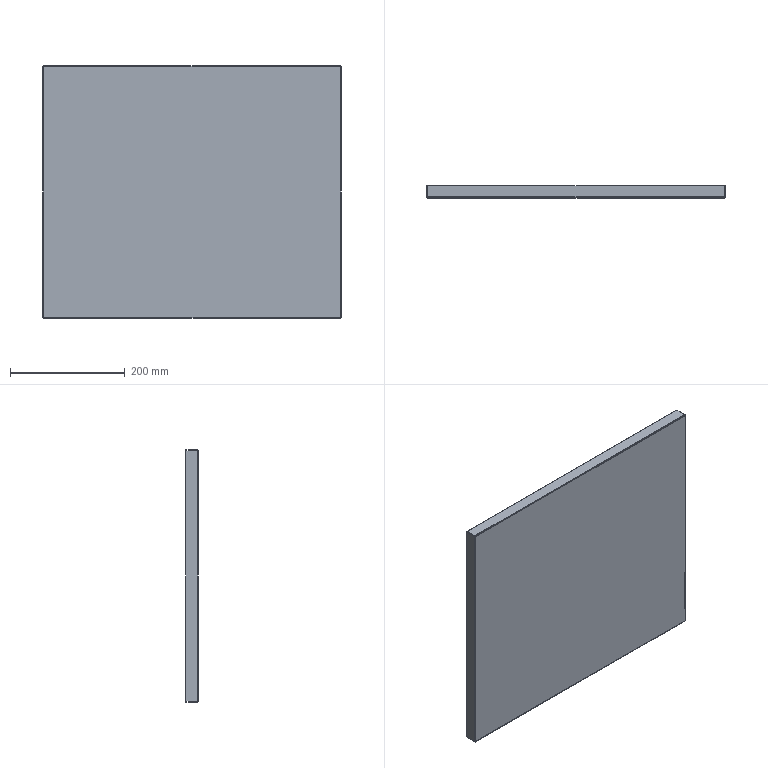Part | SolidWorks | features EdgeFlange 4, FlatPattern 1, SMBaseFlange 1, SheetMetal 1 | 1 solid | 38 faces | box 520 x 21 x 440 mm | volume 266132 mm3 | plane 30 | cylinder 8 | commonest cylinder face diameters 1 x4 3 x4
STEP:
#1=CARTESIAN_POINT('',(-258.5,1.,-218.5));
#2=VERTEX_POINT('',#1);
#3=CARTESIAN_POINT('',(-258.5,1.,218.5));
#4=VERTEX_POINT('',#3);
#5=CARTESIAN_POINT('',(-258.5,1.,-218.5));
#6=DIRECTION('',(0.,0.,1.));
#7=VECTOR('',#6,1000.);
#8=LINE('',#5,#7);
#9=EDGE_CURVE('',#2,#4,#8,.T.);
#10=ORIENTED_EDGE('',*,*,#9,.T.);
#11=CARTESIAN_POINT('',(258.5,1.,218.5));
#12=VERTEX_POINT('',#11);
#13=CARTESIAN_POINT('',(-258.5,1.,218.5));
#14=DIRECTION('',(1.,0.,0.));
#15=VECTOR('',#14,1000.);
#16=LINE('',#13,#15);
#17=EDGE_CURVE('',#4,#12,#16,.T.);
#18=ORIENTED_EDGE('',*,*,#17,.T.);
#19=CARTESIAN_POINT('',(258.5,1.,-218.5));
#20=VERTEX_POINT('',#19);
#21=CARTESIAN_POINT('',(258.5,1.,-218.5));
#22=DIRECTION('',(0.,0.,-1.));
#23=VECTOR('',#22,1000.);
#24=LINE('',#21,#23);
#25=EDGE_CURVE('',#12,#20,#24,.T.);
#26=ORIENTED_EDGE('',*,*,#25,.T.);
#27=CARTESIAN_POINT('',(-258.5,1.,-218.5));
#28=DIRECTION('',(-1.,0.,0.));
#29=VECTOR('',#28,1000.);
#30=LINE('',#27,#29);
#31=EDGE_CURVE('',#20,#2,#30,.T.);
#32=ORIENTED_EDGE('',*,*,#31,.T.);
#33=EDGE_LOOP('',(#10,#18,#26,#32));
#34=FACE_OUTER_BOUND('',#33,.T.);
#35=CARTESIAN_POINT('',(-258.5,1.,218.5));
#36=DIRECTION('',(0.,1.,0.));
#37=DIRECTION('',(0.,0.,1.));
#38=AXIS2_PLACEMENT_3D('',#35,#36,#37);
#39=PLANE('',#38);
#40=ADVANCED_FACE('',(#34),#39,.T.);
#41=CARTESIAN_POINT('',(-258.5,0.,-218.5));
#42=VERTEX_POINT('',#41);
#43=CARTESIAN_POINT('',(-258.5,0.,218.5));
#44=VERTEX_POINT('',#43);
#45=CARTESIAN_POINT('',(-258.5,0.,-218.5));
#46=DIRECTION('',(0.,0.,1.));
#47=VECTOR('',#46,1000.);
#48=LINE('',#45,#47);
#49=EDGE_CURVE('',#42,#44,#48,.T.);
#50=ORIENTED_EDGE('',*,*,#49,.F.);
#51=CARTESIAN_POINT('',(258.5,0.,-218.5));
#52=VERTEX_POINT('',#51);
#53=CARTESIAN_POINT('',(-258.5,0.,-218.5));
#54=DIRECTION('',(-1.,0.,0.));
#55=VECTOR('',#54,1000.);
#56=LINE('',#53,#55);
#57=EDGE_CURVE('',#52,#42,#56,.T.);
#58=ORIENTED_EDGE('',*,*,#57,.F.);
#59=CARTESIAN_POINT('',(258.5,0.,218.5));
#60=VERTEX_POINT('',#59);
#61=CARTESIAN_POINT('',(258.5,0.,-218.5));
#62=DIRECTION('',(0.,0.,-1.));
#63=VECTOR('',#62,1000.);
#64=LINE('',#61,#63);
#65=EDGE_CURVE('',#60,#52,#64,.T.);
#66=ORIENTED_EDGE('',*,*,#65,.F.);
#67=CARTESIAN_POINT('',(-258.5,0.,218.5));
#68=DIRECTION('',(1.,0.,0.));
#69=VECTOR('',#68,1000.);
#70=LINE('',#67,#69);
#71=EDGE_CURVE('',#44,#60,#70,.T.);
#72=ORIENTED_EDGE('',*,*,#71,.F.);
#73=EDGE_LOOP('',(#50,#58,#66,#72));
#74=FACE_OUTER_BOUND('',#73,.T.);
#75=CARTESIAN_POINT('',(-258.5,0.,218.5));
#76=DIRECTION('',(0.,1.,0.));
#77=DIRECTION('',(0.,0.,1.));
#78=AXIS2_PLACEMENT_3D('',#75,#76,#77);
#79=PLANE('',#78);
#80=ADVANCED_FACE('',(#74),#79,.F.);
#81=CARTESIAN_POINT('',(-259.,1.5,-218.5));
#82=VERTEX_POINT('',#81);
#83=CARTESIAN_POINT('',(-260.,1.5,-218.5));
#84=VERTEX_POINT('',#83);
#85=CARTESIAN_POINT('',(-260.,1.5,-218.5));
#86=DIRECTION('',(-1.,0.,0.));
#87=VECTOR('',#86,1000.);
#88=LINE('',#85,#87);
#89=EDGE_CURVE('',#82,#84,#88,.T.);
#90=ORIENTED_EDGE('',*,*,#89,.F.);
#91=CARTESIAN_POINT('',(-258.5,1.5,-218.5));
#92=DIRECTION('',(0.,0.,-1.));
#93=DIRECTION('',(0.,-1.,0.));
#94=AXIS2_PLACEMENT_3D('',#91,#92,#93);
#95=CIRCLE('',#94,0.5);
#96=EDGE_CURVE('',#2,#82,#95,.T.);
#97=ORIENTED_EDGE('',*,*,#96,.F.);
#98=CARTESIAN_POINT('',(-258.5,1.,-218.5));
#99=DIRECTION('',(0.,-1.,0.));
#100=VECTOR('',#99,1000.);
#101=LINE('',#98,#100);
#102=EDGE_CURVE('',#2,#42,#101,.T.);
#103=ORIENTED_EDGE('',*,*,#102,.T.);
#104=CARTESIAN_POINT('',(-258.5,1.5,-218.5));
#105=DIRECTION('',(0.,0.,-1.));
#106=DIRECTION('',(0.,-1.,0.));
#107=AXIS2_PLACEMENT_3D('',#104,#105,#106);
#108=CIRCLE('',#107,1.5);
#109=EDGE_CURVE('',#42,#84,#108,.T.);
#110=ORIENTED_EDGE('',*,*,#109,.T.);
#111=EDGE_LOOP('',(#90,#97,#103,#110));
#112=FACE_OUTER_BOUND('',#111,.T.);
#113=CARTESIAN_POINT('',(-258.5,1.5,-218.5));
#114=DIRECTION('',(0.,0.,-1.));
#115=DIRECTION('',(0.,1.,0.));
#116=AXIS2_PLACEMENT_3D('',#113,#114,#115);
#117=PLANE('',#116);
#118=ADVANCED_FACE('',(#112),#117,.T.);
#119=ORIENTED_EDGE('',*,*,#49,.T.);
#120=CARTESIAN_POINT('',(-260.,1.5,218.5));
#121=VERTEX_POINT('',#120);
#122=CARTESIAN_POINT('',(-258.5,1.5,218.5));
#123=DIRECTION('',(0.,0.,1.));
#124=DIRECTION('',(0.,-1.,0.));
#125=AXIS2_PLACEMENT_3D('',#122,#123,#124);
#126=CIRCLE('',#125,1.5);
#127=EDGE_CURVE('',#121,#44,#126,.T.);
#128=ORIENTED_EDGE('',*,*,#127,.F.);
#129=CARTESIAN_POINT('',(-260.,1.5,-218.5));
#130=DIRECTION('',(0.,0.,-1.));
#131=VECTOR('',#130,1000.);
#132=LINE('',#129,#131);
#133=EDGE_CURVE('',#121,#84,#132,.T.);
#134=ORIENTED_EDGE('',*,*,#133,.T.);
#135=ORIENTED_EDGE('',*,*,#109,.F.);
#136=EDGE_LOOP('',(#119,#128,#134,#135));
#137=FACE_OUTER_BOUND('',#136,.T.);
#138=CARTESIAN_POINT('',(-258.5,1.5,218.5));
#139=DIRECTION('',(0.,0.,1.));
#140=DIRECTION('',(-1.,0.,0.));
#141=AXIS2_PLACEMENT_3D('',#138,#139,#140);
#142=CYLINDRICAL_SURFACE('',#141,1.5);
#143=ADVANCED_FACE('',(#137),#142,.T.);
#144=CARTESIAN_POINT('',(-259.,1.5,218.5));
#145=VERTEX_POINT('',#144);
#146=CARTESIAN_POINT('',(-258.5,1.5,218.5));
#147=DIRECTION('',(0.,0.,1.));
#148=DIRECTION('',(0.,-1.,0.));
#149=AXIS2_PLACEMENT_3D('',#146,#147,#148);
#150=CIRCLE('',#149,0.5);
#151=EDGE_CURVE('',#145,#4,#150,.T.);
#152=ORIENTED_EDGE('',*,*,#151,.F.);
#153=CARTESIAN_POINT('',(-259.,1.5,218.5));
#154=DIRECTION('',(-1.,0.,0.));
#155=VECTOR('',#154,1000.);
#156=LINE('',#153,#155);
#157=EDGE_CURVE('',#145,#121,#156,.T.);
#158=ORIENTED_EDGE('',*,*,#157,.T.);
#159=ORIENTED_EDGE('',*,*,#127,.T.);
#160=CARTESIAN_POINT('',(-258.5,1.,218.5));
#161=DIRECTION('',(0.,-1.,0.));
#162=VECTOR('',#161,1000.);
#163=LINE('',#160,#162);
#164=EDGE_CURVE('',#4,#44,#163,.T.);
#165=ORIENTED_EDGE('',*,*,#164,.F.);
#166=EDGE_LOOP('',(#152,#158,#159,#165));
#167=FACE_OUTER_BOUND('',#166,.T.);
#168=CARTESIAN_POINT('',(-258.5,1.5,218.5));
#169=DIRECTION('',(0.,0.,-1.));
#170=DIRECTION('',(0.,1.,0.));
#171=AXIS2_PLACEMENT_3D('',#168,#169,#170);
#172=PLANE('',#171);
#173=ADVANCED_FACE('',(#167),#172,.F.);
#174=ORIENTED_EDGE('',*,*,#9,.F.);
#175=ORIENTED_EDGE('',*,*,#96,.T.);
#176=CARTESIAN_POINT('',(-259.,1.5,-218.5));
#177=DIRECTION('',(0.,0.,1.));
#178=VECTOR('',#177,1000.);
#179=LINE('',#176,#178);
#180=EDGE_CURVE('',#82,#145,#179,.T.);
#181=ORIENTED_EDGE('',*,*,#180,.T.);
#182=ORIENTED_EDGE('',*,*,#151,.T.);
#183=EDGE_LOOP('',(#174,#175,#181,#182));
#184=FACE_OUTER_BOUND('',#183,.T.);
#185=CARTESIAN_POINT('',(-258.5,1.5,218.5));
#186=DIRECTION('',(0.,0.,1.));
#187=DIRECTION('',(-1.,0.,0.));
#188=AXIS2_PLACEMENT_3D('',#185,#186,#187);
#189=CYLINDRICAL_SURFACE('',#188,0.5);
#190=ADVANCED_FACE('',(#184),#189,.F.);
#191=CARTESIAN_POINT('',(-260.,21.,218.5));
#192=VERTEX_POINT('',#191);
#193=CARTESIAN_POINT('',(-260.,1.,218.5));
#194=DIRECTION('',(0.,-1.,0.));
#195=VECTOR('',#194,1000.);
#196=LINE('',#193,#195);
#197=EDGE_CURVE('',#192,#121,#196,.T.);
#198=ORIENTED_EDGE('',*,*,#197,.T.);
#199=ORIENTED_EDGE('',*,*,#157,.F.);
#200=CARTESIAN_POINT('',(-259.,21.,218.5));
#201=VERTEX_POINT('',#200);
#202=CARTESIAN_POINT('',(-259.,1.,218.5));
#203=DIRECTION('',(0.,-1.,0.));
#204=VECTOR('',#203,1000.);
#205=LINE('',#202,#204);
#206=EDGE_CURVE('',#201,#145,#205,.T.);
#207=ORIENTED_EDGE('',*,*,#206,.F.);
#208=CARTESIAN_POINT('',(-260.,21.,218.5));
#209=DIRECTION('',(1.,0.,0.));
#210=VECTOR('',#209,1000.);
#211=LINE('',#208,#210);
#212=EDGE_CURVE('',#192,#201,#211,.T.);
#213=ORIENTED_EDGE('',*,*,#212,.F.);
#214=EDGE_LOOP('',(#198,#199,#207,#213));
#215=FACE_OUTER_BOUND('',#214,.T.);
#216=CARTESIAN_POINT('',(-260.,1.,218.5));
#217=DIRECTION('',(0.,0.,1.));
#218=DIRECTION('',(0.,-1.,0.));
#219=AXIS2_PLACEMENT_3D('',#216,#217,#218);
#220=PLANE('',#219);
#221=ADVANCED_FACE('',(#215),#220,.T.);
#222=CARTESIAN_POINT('',(-259.,21.,-218.5));
#223=VERTEX_POINT('',#222);
#224=CARTESIAN_POINT('',(-259.,1.,-218.5));
#225=DIRECTION('',(0.,1.,0.));
#226=VECTOR('',#225,1000.);
#227=LINE('',#224,#226);
#228=EDGE_CURVE('',#82,#223,#227,.T.);
#229=ORIENTED_EDGE('',*,*,#228,.F.);
#230=ORIENTED_EDGE('',*,*,#89,.T.);
#231=CARTESIAN_POINT('',(-260.,21.,-218.5));
#232=VERTEX_POINT('',#231);
#233=CARTESIAN_POINT('',(-260.,21.,-218.5));
#234=DIRECTION('',(0.,1.,0.));
#235=VECTOR('',#234,1000.);
#236=LINE('',#233,#235);
#237=EDGE_CURVE('',#84,#232,#236,.T.);
#238=ORIENTED_EDGE('',*,*,#237,.T.);
#239=CARTESIAN_POINT('',(-260.,21.,-218.5));
#240=DIRECTION('',(1.,0.,0.));
#241=VECTOR('',#240,1000.);
#242=LINE('',#239,#241);
#243=EDGE_CURVE('',#232,#223,#242,.T.);
#244=ORIENTED_EDGE('',*,*,#243,.T.);
#245=EDGE_LOOP('',(#229,#230,#238,#244));
#246=FACE_OUTER_BOUND('',#245,.T.);
#247=CARTESIAN_POINT('',(-260.,21.,-218.5));
#248=DIRECTION('',(0.,0.,-1.));
#249=DIRECTION('',(0.,1.,0.));
#250=AXIS2_PLACEMENT_3D('',#247,#248,#249);
#251=PLANE('',#250);
#252=ADVANCED_FACE('',(#246),#251,.T.);
#253=ORIENTED_EDGE('',*,*,#133,.F.);
#254=ORIENTED_EDGE('',*,*,#197,.F.);
#255=CARTESIAN_POINT('',(-260.,21.,218.5));
#256=DIRECTION('',(0.,0.,1.));
#257=VECTOR('',#256,1000.);
#258=LINE('',#255,#257);
#259=EDGE_CURVE('',#232,#192,#258,.T.);
#260=ORIENTED_EDGE('',*,*,#259,.F.);
#261=ORIENTED_EDGE('',*,*,#237,.F.);
#262=EDGE_LOOP('',(#253,#254,#260,#261));
#263=FACE_OUTER_BOUND('',#262,.T.);
#264=CARTESIAN_POINT('',(-260.,1.,-218.5));
#265=DIRECTION('',(1.,0.,0.));
#266=DIRECTION('',(0.,1.,0.));
#267=AXIS2_PLACEMENT_3D('',#264,#265,#266);
#268=PLANE('',#267);
#269=ADVANCED_FACE('',(#263),#268,.F.);
#270=ORIENTED_EDGE('',*,*,#206,.T.);
#271=ORIENTED_EDGE('',*,*,#180,.F.);
#272=ORIENTED_EDGE('',*,*,#228,.T.);
#273=CARTESIAN_POINT('',(-259.,21.,-218.5));
#274=DIRECTION('',(0.,0.,1.));
#275=VECTOR('',#274,1000.);
#276=LINE('',#273,#275);
#277=EDGE_CURVE('',#223,#201,#276,.T.);
#278=ORIENTED_EDGE('',*,*,#277,.T.);
#279=EDGE_LOOP('',(#270,#271,#272,#278));
#280=FACE_OUTER_BOUND('',#279,.T.);
#281=CARTESIAN_POINT('',(-259.,1.,-218.5));
#282=DIRECTION('',(1.,0.,0.));
#283=DIRECTION('',(0.,1.,0.));
#284=AXIS2_PLACEMENT_3D('',#281,#282,#283);
#285=PLANE('',#284);
#286=ADVANCED_FACE('',(#280),#285,.T.);
#287=ORIENTED_EDGE('',*,*,#277,.F.);
#288=ORIENTED_EDGE('',*,*,#243,.F.);
#289=ORIENTED_EDGE('',*,*,#259,.T.);
#290=ORIENTED_EDGE('',*,*,#212,.T.);
#291=EDGE_LOOP('',(#287,#288,#289,#290));
#292=FACE_OUTER_BOUND('',#291,.T.);
#293=CARTESIAN_POINT('',(-260.,21.,218.5));
#294=DIRECTION('',(0.,1.,0.));
#295=DIRECTION('',(-1.,0.,0.));
#296=AXIS2_PLACEMENT_3D('',#293,#294,#295);
#297=PLANE('',#296);
#298=ADVANCED_FACE('',(#292),#297,.T.);
#299=CARTESIAN_POINT('',(259.,1.5,218.5));
#300=VERTEX_POINT('',#299);
#301=CARTESIAN_POINT('',(260.,1.5,218.5));
#302=VERTEX_POINT('',#301);
#303=CARTESIAN_POINT('',(260.,1.5,218.5));
#304=DIRECTION('',(1.,0.,0.));
#305=VECTOR('',#304,1000.);
#306=LINE('',#303,#305);
#307=EDGE_CURVE('',#300,#302,#306,.T.);
#308=ORIENTED_EDGE('',*,*,#307,.F.);
#309=CARTESIAN_POINT('',(258.5,1.5,218.5));
#310=DIRECTION('',(0.,0.,1.));
#311=DIRECTION('',(0.,1.,0.));
#312=AXIS2_PLACEMENT_3D('',#309,#310,#311);
#313=CIRCLE('',#312,0.5);
#314=EDGE_CURVE('',#12,#300,#313,.T.);
#315=ORIENTED_EDGE('',*,*,#314,.F.);
#316=CARTESIAN_POINT('',(258.5,1.,218.5));
#317=DIRECTION('',(0.,-1.,0.));
#318=VECTOR('',#317,1000.);
#319=LINE('',#316,#318);
#320=EDGE_CURVE('',#12,#60,#319,.T.);
#321=ORIENTED_EDGE('',*,*,#320,.T.);
#322=CARTESIAN_POINT('',(258.5,1.5,218.5));
#323=DIRECTION('',(0.,0.,1.));
#324=DIRECTION('',(0.,1.,0.));
#325=AXIS2_PLACEMENT_3D('',#322,#323,#324);
#326=CIRCLE('',#325,1.5);
#327=EDGE_CURVE('',#60,#302,#326,.T.);
#328=ORIENTED_EDGE('',*,*,#327,.T.);
#329=EDGE_LOOP('',(#308,#315,#321,#328));
#330=FACE_OUTER_BOUND('',#329,.T.);
#331=CARTESIAN_POINT('',(258.5,1.5,218.5));
#332=DIRECTION('',(0.,0.,1.));
#333=DIRECTION('',(0.,-1.,0.));
#334=AXIS2_PLACEMENT_3D('',#331,#332,#333);
#335=PLANE('',#334);
#336=ADVANCED_FACE('',(#330),#335,.T.);
#337=ORIENTED_EDGE('',*,*,#65,.T.);
#338=CARTESIAN_POINT('',(260.,1.5,-218.5));
#339=VERTEX_POINT('',#338);
#340=CARTESIAN_POINT('',(258.5,1.5,-218.5));
#341=DIRECTION('',(0.,0.,-1.));
#342=DIRECTION('',(0.,1.,0.));
#343=AXIS2_PLACEMENT_3D('',#340,#341,#342);
#344=CIRCLE('',#343,1.5);
#345=EDGE_CURVE('',#339,#52,#344,.T.);
#346=ORIENTED_EDGE('',*,*,#345,.F.);
#347=CARTESIAN_POINT('',(260.,1.5,-218.5));
#348=DIRECTION('',(0.,0.,-1.));
#349=VECTOR('',#348,1000.);
#350=LINE('',#347,#349);
#351=EDGE_CURVE('',#302,#339,#350,.T.);
#352=ORIENTED_EDGE('',*,*,#351,.F.);
#353=ORIENTED_EDGE('',*,*,#327,.F.);
#354=EDGE_LOOP('',(#337,#346,#352,#353));
#355=FACE_OUTER_BOUND('',#354,.T.);
#356=CARTESIAN_POINT('',(258.5,1.5,-218.5));
#357=DIRECTION('',(0.,0.,-1.));
#358=DIRECTION('',(1.,0.,0.));
#359=AXIS2_PLACEMENT_3D('',#356,#357,#358);
#360=CYLINDRICAL_SURFACE('',#359,1.5);
#361=ADVANCED_FACE('',(#355),#360,.T.);
#362=CARTESIAN_POINT('',(259.,1.5,-218.5));
#363=VERTEX_POINT('',#362);
#364=CARTESIAN_POINT('',(258.5,1.5,-218.5));
#365=DIRECTION('',(0.,0.,-1.));
#366=DIRECTION('',(0.,1.,0.));
#367=AXIS2_PLACEMENT_3D('',#364,#365,#366);
#368=CIRCLE('',#367,0.5);
#369=EDGE_CURVE('',#363,#20,#368,.T.);
#370=ORIENTED_EDGE('',*,*,#369,.F.);
#371=CARTESIAN_POINT('',(259.,1.5,-218.5));
#372=DIRECTION('',(1.,0.,0.));
#373=VECTOR('',#372,1000.);
#374=LINE('',#371,#373);
#375=EDGE_CURVE('',#363,#339,#374,.T.);
#376=ORIENTED_EDGE('',*,*,#375,.T.);
#377=ORIENTED_EDGE('',*,*,#345,.T.);
#378=CARTESIAN_POINT('',(258.5,1.,-218.5));
#379=DIRECTION('',(0.,-1.,0.));
#380=VECTOR('',#379,1000.);
#381=LINE('',#378,#380);
#382=EDGE_CURVE('',#20,#52,#381,.T.);
#383=ORIENTED_EDGE('',*,*,#382,.F.);
#384=EDGE_LOOP('',(#370,#376,#377,#383));
#385=FACE_OUTER_BOUND('',#384,.T.);
#386=CARTESIAN_POINT('',(258.5,1.5,-218.5));
#387=DIRECTION('',(0.,0.,1.));
#388=DIRECTION('',(0.,-1.,0.));
#389=AXIS2_PLACEMENT_3D('',#386,#387,#388);
#390=PLANE('',#389);
#391=ADVANCED_FACE('',(#385),#390,.F.);
#392=ORIENTED_EDGE('',*,*,#25,.F.);
#393=ORIENTED_EDGE('',*,*,#314,.T.);
#394=CARTESIAN_POINT('',(259.,1.5,218.5));
#395=DIRECTION('',(0.,0.,-1.));
#396=VECTOR('',#395,1000.);
#397=LINE('',#394,#396);
#398=EDGE_CURVE('',#300,#363,#397,.T.);
#399=ORIENTED_EDGE('',*,*,#398,.T.);
#400=ORIENTED_EDGE('',*,*,#369,.T.);
#401=EDGE_LOOP('',(#392,#393,#399,#400));
#402=FACE_OUTER_BOUND('',#401,.T.);
#403=CARTESIAN_POINT('',(258.5,1.5,-218.5));
#404=DIRECTION('',(0.,0.,-1.));
#405=DIRECTION('',(1.,0.,0.));
#406=AXIS2_PLACEMENT_3D('',#403,#404,#405);
#407=CYLINDRICAL_SURFACE('',#406,0.5);
#408=ADVANCED_FACE('',(#402),#407,.F.);
#409=CARTESIAN_POINT('',(260.,21.,-218.5));
#410=VERTEX_POINT('',#409);
#411=CARTESIAN_POINT('',(260.,1.,-218.5));
#412=DIRECTION('',(0.,-1.,0.));
#413=VECTOR('',#412,1000.);
#414=LINE('',#411,#413);
#415=EDGE_CURVE('',#410,#339,#414,.T.);
#416=ORIENTED_EDGE('',*,*,#415,.T.);
#417=ORIENTED_EDGE('',*,*,#375,.F.);
#418=CARTESIAN_POINT('',(259.,21.,-218.5));
#419=VERTEX_POINT('',#418);
#420=CARTESIAN_POINT('',(259.,1.,-218.5));
#421=DIRECTION('',(0.,-1.,0.));
#422=VECTOR('',#421,1000.);
#423=LINE('',#420,#422);
#424=EDGE_CURVE('',#419,#363,#423,.T.);
#425=ORIENTED_EDGE('',*,*,#424,.F.);
#426=CARTESIAN_POINT('',(260.,21.,-218.5));
#427=DIRECTION('',(-1.,0.,0.));
#428=VECTOR('',#427,1000.);
#429=LINE('',#426,#428);
#430=EDGE_CURVE('',#410,#419,#429,.T.);
#431=ORIENTED_EDGE('',*,*,#430,.F.);
#432=EDGE_LOOP('',(#416,#417,#425,#431));
#433=FACE_OUTER_BOUND('',#432,.T.);
#434=CARTESIAN_POINT('',(260.,1.,-218.5));
#435=DIRECTION('',(0.,0.,-1.));
#436=DIRECTION('',(-1.,0.,0.));
#437=AXIS2_PLACEMENT_3D('',#434,#435,#436);
#438=PLANE('',#437);
#439=ADVANCED_FACE('',(#433),#438,.T.);
#440=CARTESIAN_POINT('',(259.,21.,218.5));
#441=VERTEX_POINT('',#440);
#442=CARTESIAN_POINT('',(259.,1.,218.5));
#443=DIRECTION('',(0.,1.,0.));
#444=VECTOR('',#443,1000.);
#445=LINE('',#442,#444);
#446=EDGE_CURVE('',#300,#441,#445,.T.);
#447=ORIENTED_EDGE('',*,*,#446,.F.);
#448=ORIENTED_EDGE('',*,*,#307,.T.);
#449=CARTESIAN_POINT('',(260.,21.,218.5));
#450=VERTEX_POINT('',#449);
#451=CARTESIAN_POINT('',(260.,21.,218.5));
#452=DIRECTION('',(0.,1.,0.));
#453=VECTOR('',#452,1000.);
#454=LINE('',#451,#453);
#455=EDGE_CURVE('',#302,#450,#454,.T.);
#456=ORIENTED_EDGE('',*,*,#455,.T.);
#457=CARTESIAN_POINT('',(260.,21.,218.5));
#458=DIRECTION('',(-1.,0.,0.));
#459=VECTOR('',#458,1000.);
#460=LINE('',#457,#459);
#461=EDGE_CURVE('',#450,#441,#460,.T.);
#462=ORIENTED_EDGE('',*,*,#461,.T.);
#463=EDGE_LOOP('',(#447,#448,#456,#462));
#464=FACE_OUTER_BOUND('',#463,.T.);
#465=CARTESIAN_POINT('',(260.,21.,218.5));
#466=DIRECTION('',(0.,0.,1.));
#467=DIRECTION('',(0.,-1.,0.));
#468=AXIS2_PLACEMENT_3D('',#465,#466,#467);
#469=PLANE('',#468);
#470=ADVANCED_FACE('',(#464),#469,.T.);
#471=ORIENTED_EDGE('',*,*,#455,.F.);
#472=ORIENTED_EDGE('',*,*,#351,.T.);
#473=ORIENTED_EDGE('',*,*,#415,.F.);
#474=CARTESIAN_POINT('',(260.,21.,-218.5));
#475=DIRECTION('',(0.,0.,-1.));
#476=VECTOR('',#475,1000.);
#477=LINE('',#474,#476);
#478=EDGE_CURVE('',#450,#410,#477,.T.);
#479=ORIENTED_EDGE('',*,*,#478,.F.);
#480=EDGE_LOOP('',(#471,#472,#473,#479));
#481=FACE_OUTER_BOUND('',#480,.T.);
#482=CARTESIAN_POINT('',(260.,1.,-218.5));
#483=DIRECTION('',(1.,0.,0.));
#484=DIRECTION('',(0.,1.,0.));
#485=AXIS2_PLACEMENT_3D('',#482,#483,#484);
#486=PLANE('',#485);
#487=ADVANCED_FACE('',(#481),#486,.T.);
#488=ORIENTED_EDGE('',*,*,#398,.F.);
#489=ORIENTED_EDGE('',*,*,#446,.T.);
#490=CARTESIAN_POINT('',(259.,21.,-218.5));
#491=DIRECTION('',(0.,0.,-1.));
#492=VECTOR('',#491,1000.);
#493=LINE('',#490,#492);
#494=EDGE_CURVE('',#441,#419,#493,.T.);
#495=ORIENTED_EDGE('',*,*,#494,.T.);
#496=ORIENTED_EDGE('',*,*,#424,.T.);
#497=EDGE_LOOP('',(#488,#489,#495,#496));
#498=FACE_OUTER_BOUND('',#497,.T.);
#499=CARTESIAN_POINT('',(259.,1.,-218.5));
#500=DIRECTION('',(1.,0.,0.));
#501=DIRECTION('',(0.,1.,0.));
#502=AXIS2_PLACEMENT_3D('',#499,#500,#501);
#503=PLANE('',#502);
#504=ADVANCED_FACE('',(#498),#503,.F.);
#505=ORIENTED_EDGE('',*,*,#494,.F.);
#506=ORIENTED_EDGE('',*,*,#461,.F.);
#507=ORIENTED_EDGE('',*,*,#478,.T.);
#508=ORIENTED_EDGE('',*,*,#430,.T.);
#509=EDGE_LOOP('',(#505,#506,#507,#508));
#510=FACE_OUTER_BOUND('',#509,.T.);
#511=CARTESIAN_POINT('',(260.,21.,-218.5));
#512=DIRECTION('',(0.,1.,0.));
#513=DIRECTION('',(-1.,0.,0.));
#514=AXIS2_PLACEMENT_3D('',#511,#512,#513);
#515=PLANE('',#514);
#516=ADVANCED_FACE('',(#510),#515,.T.);
#517=CARTESIAN_POINT('',(258.5,1.5,-219.));
#518=VERTEX_POINT('',#517);
#519=CARTESIAN_POINT('',(258.5,1.5,-220.));
#520=VERTEX_POINT('',#519);
#521=CARTESIAN_POINT('',(258.5,1.5,-220.));
#522=DIRECTION('',(0.,0.,-1.));
#523=VECTOR('',#522,1000.);
#524=LINE('',#521,#523);
#525=EDGE_CURVE('',#518,#520,#524,.T.);
#526=ORIENTED_EDGE('',*,*,#525,.F.);
#527=CARTESIAN_POINT('',(258.5,1.5,-218.5));
#528=DIRECTION('',(1.,0.,0.));
#529=DIRECTION('',(0.,0.,1.));
#530=AXIS2_PLACEMENT_3D('',#527,#528,#529);
#531=CIRCLE('',#530,0.5);
#532=EDGE_CURVE('',#20,#518,#531,.T.);
#533=ORIENTED_EDGE('',*,*,#532,.F.);
#534=ORIENTED_EDGE('',*,*,#382,.T.);
#535=CARTESIAN_POINT('',(258.5,1.5,-218.5));
#536=DIRECTION('',(1.,0.,0.));
#537=DIRECTION('',(0.,0.,1.));
#538=AXIS2_PLACEMENT_3D('',#535,#536,#537);
#539=CIRCLE('',#538,1.5);
#540=EDGE_CURVE('',#52,#520,#539,.T.);
#541=ORIENTED_EDGE('',*,*,#540,.T.);
#542=EDGE_LOOP('',(#526,#533,#534,#541));
#543=FACE_OUTER_BOUND('',#542,.T.);
#544=CARTESIAN_POINT('',(258.5,1.5,-218.5));
#545=DIRECTION('',(1.,0.,0.));
#546=DIRECTION('',(0.,0.,-1.));
#547=AXIS2_PLACEMENT_3D('',#544,#545,#546);
#548=PLANE('',#547);
#549=ADVANCED_FACE('',(#543),#548,.T.);
#550=ORIENTED_EDGE('',*,*,#57,.T.);
#551=CARTESIAN_POINT('',(-258.5,1.5,-220.));
#552=VERTEX_POINT('',#551);
#553=CARTESIAN_POINT('',(-258.5,1.5,-218.5));
#554=DIRECTION('',(-1.,0.,0.));
#555=DIRECTION('',(0.,0.,1.));
#556=AXIS2_PLACEMENT_3D('',#553,#554,#555);
#557=CIRCLE('',#556,1.5);
#558=EDGE_CURVE('',#552,#42,#557,.T.);
#559=ORIENTED_EDGE('',*,*,#558,.F.);
#560=CARTESIAN_POINT('',(258.5,1.5,-220.));
#561=DIRECTION('',(1.,0.,0.));
#562=VECTOR('',#561,1000.);
#563=LINE('',#560,#562);
#564=EDGE_CURVE('',#552,#520,#563,.T.);
#565=ORIENTED_EDGE('',*,*,#564,.T.);
#566=ORIENTED_EDGE('',*,*,#540,.F.);
#567=EDGE_LOOP('',(#550,#559,#565,#566));
#568=FACE_OUTER_BOUND('',#567,.T.);
#569=CARTESIAN_POINT('',(-258.5,1.5,-218.5));
#570=DIRECTION('',(-1.,0.,0.));
#571=DIRECTION('',(0.,0.,-1.));
#572=AXIS2_PLACEMENT_3D('',#569,#570,#571);
#573=CYLINDRICAL_SURFACE('',#572,1.5);
#574=ADVANCED_FACE('',(#568),#573,.T.);
#575=CARTESIAN_POINT('',(-258.5,1.5,-219.));
#576=VERTEX_POINT('',#575);
#577=CARTESIAN_POINT('',(-258.5,1.5,-218.5));
#578=DIRECTION('',(-1.,0.,0.));
#579=DIRECTION('',(0.,0.,1.));
#580=AXIS2_PLACEMENT_3D('',#577,#578,#579);
#581=CIRCLE('',#580,0.5);
#582=EDGE_CURVE('',#576,#2,#581,.T.);
#583=ORIENTED_EDGE('',*,*,#582,.F.);
#584=CARTESIAN_POINT('',(-258.5,1.5,-219.));
#585=DIRECTION('',(0.,0.,-1.));
#586=VECTOR('',#585,1000.);
#587=LINE('',#584,#586);
#588=EDGE_CURVE('',#576,#552,#587,.T.);
#589=ORIENTED_EDGE('',*,*,#588,.T.);
#590=ORIENTED_EDGE('',*,*,#558,.T.);
#591=ORIENTED_EDGE('',*,*,#102,.F.);
#592=EDGE_LOOP('',(#583,#589,#590,#591));
#593=FACE_OUTER_BOUND('',#592,.T.);
#594=CARTESIAN_POINT('',(-258.5,1.5,-218.5));
#595=DIRECTION('',(1.,0.,0.));
#596=DIRECTION('',(0.,0.,-1.));
#597=AXIS2_PLACEMENT_3D('',#594,#595,#596);
#598=PLANE('',#597);
#599=ADVANCED_FACE('',(#593),#598,.F.);
#600=ORIENTED_EDGE('',*,*,#31,.F.);
#601=ORIENTED_EDGE('',*,*,#532,.T.);
#602=CARTESIAN_POINT('',(258.5,1.5,-219.));
#603=DIRECTION('',(-1.,0.,0.));
#604=VECTOR('',#603,1000.);
#605=LINE('',#602,#604);
#606=EDGE_CURVE('',#518,#576,#605,.T.);
#607=ORIENTED_EDGE('',*,*,#606,.T.);
#608=ORIENTED_EDGE('',*,*,#582,.T.);
#609=EDGE_LOOP('',(#600,#601,#607,#608));
#610=FACE_OUTER_BOUND('',#609,.T.);
#611=CARTESIAN_POINT('',(-258.5,1.5,-218.5));
#612=DIRECTION('',(-1.,0.,0.));
#613=DIRECTION('',(0.,0.,-1.));
#614=AXIS2_PLACEMENT_3D('',#611,#612,#613);
#615=CYLINDRICAL_SURFACE('',#614,0.5);
#616=ADVANCED_FACE('',(#610),#615,.F.);
#617=CARTESIAN_POINT('',(-258.5,21.,-220.));
#618=VERTEX_POINT('',#617);
#619=CARTESIAN_POINT('',(-258.5,1.,-220.));
#620=DIRECTION('',(0.,-1.,0.));
#621=VECTOR('',#620,1000.);
#622=LINE('',#619,#621);
#623=EDGE_CURVE('',#618,#552,#622,.T.);
#624=ORIENTED_EDGE('',*,*,#623,.T.);
#625=ORIENTED_EDGE('',*,*,#588,.F.);
#626=CARTESIAN_POINT('',(-258.5,21.,-219.));
#627=VERTEX_POINT('',#626);
#628=CARTESIAN_POINT('',(-258.5,1.,-219.));
#629=DIRECTION('',(0.,-1.,0.));
#630=VECTOR('',#629,1000.);
#631=LINE('',#628,#630);
#632=EDGE_CURVE('',#627,#576,#631,.T.);
#633=ORIENTED_EDGE('',*,*,#632,.F.);
#634=CARTESIAN_POINT('',(-258.5,21.,-220.));
#635=DIRECTION('',(0.,0.,1.));
#636=VECTOR('',#635,1000.);
#637=LINE('',#634,#636);
#638=EDGE_CURVE('',#618,#627,#637,.T.);
#639=ORIENTED_EDGE('',*,*,#638,.F.);
#640=EDGE_LOOP('',(#624,#625,#633,#639));
#641=FACE_OUTER_BOUND('',#640,.T.);
#642=CARTESIAN_POINT('',(-258.5,1.,-220.));
#643=DIRECTION('',(-1.,0.,0.));
#644=DIRECTION('',(0.,-1.,0.));
#645=AXIS2_PLACEMENT_3D('',#642,#643,#644);
#646=PLANE('',#645);
#647=ADVANCED_FACE('',(#641),#646,.T.);
#648=CARTESIAN_POINT('',(258.5,21.,-219.));
#649=VERTEX_POINT('',#648);
#650=CARTESIAN_POINT('',(258.5,1.,-219.));
#651=DIRECTION('',(0.,1.,0.));
#652=VECTOR('',#651,1000.);
#653=LINE('',#650,#652);
#654=EDGE_CURVE('',#518,#649,#653,.T.);
#655=ORIENTED_EDGE('',*,*,#654,.F.);
#656=ORIENTED_EDGE('',*,*,#525,.T.);
#657=CARTESIAN_POINT('',(258.5,21.,-220.));
#658=VERTEX_POINT('',#657);
#659=CARTESIAN_POINT('',(258.5,21.,-220.));
#660=DIRECTION('',(0.,1.,0.));
#661=VECTOR('',#660,1000.);
#662=LINE('',#659,#661);
#663=EDGE_CURVE('',#520,#658,#662,.T.);
#664=ORIENTED_EDGE('',*,*,#663,.T.);
#665=CARTESIAN_POINT('',(258.5,21.,-220.));
#666=DIRECTION('',(0.,0.,1.));
#667=VECTOR('',#666,1000.);
#668=LINE('',#665,#667);
#669=EDGE_CURVE('',#658,#649,#668,.T.);
#670=ORIENTED_EDGE('',*,*,#669,.T.);
#671=EDGE_LOOP('',(#655,#656,#664,#670));
#672=FACE_OUTER_BOUND('',#671,.T.);
#673=CARTESIAN_POINT('',(258.5,21.,-220.));
#674=DIRECTION('',(1.,0.,0.));
#675=DIRECTION('',(0.,0.,-1.));
#676=AXIS2_PLACEMENT_3D('',#673,#674,#675);
#677=PLANE('',#676);
#678=ADVANCED_FACE('',(#672),#677,.T.);
#679=ORIENTED_EDGE('',*,*,#564,.F.);
#680=ORIENTED_EDGE('',*,*,#623,.F.);
#681=CARTESIAN_POINT('',(-258.5,21.,-220.));
#682=DIRECTION('',(-1.,0.,0.));
#683=VECTOR('',#682,1000.);
#684=LINE('',#681,#683);
#685=EDGE_CURVE('',#658,#618,#684,.T.);
#686=ORIENTED_EDGE('',*,*,#685,.F.);
#687=ORIENTED_EDGE('',*,*,#663,.F.);
#688=EDGE_LOOP('',(#679,#680,#686,#687));
#689=FACE_OUTER_BOUND('',#688,.T.);
#690=CARTESIAN_POINT('',(258.5,1.,-220.));
#691=DIRECTION('',(0.,0.,1.));
#692=DIRECTION('',(1.,0.,0.));
#693=AXIS2_PLACEMENT_3D('',#690,#691,#692);
#694=PLANE('',#693);
#695=ADVANCED_FACE('',(#689),#694,.F.);
#696=ORIENTED_EDGE('',*,*,#632,.T.);
#697=ORIENTED_EDGE('',*,*,#606,.F.);
#698=ORIENTED_EDGE('',*,*,#654,.T.);
#699=CARTESIAN_POINT('',(258.5,21.,-219.));
#700=DIRECTION('',(-1.,0.,0.));
#701=VECTOR('',#700,1000.);
#702=LINE('',#699,#701);
#703=EDGE_CURVE('',#649,#627,#702,.T.);
#704=ORIENTED_EDGE('',*,*,#703,.T.);
#705=EDGE_LOOP('',(#696,#697,#698,#704));
#706=FACE_OUTER_BOUND('',#705,.T.);
#707=CARTESIAN_POINT('',(258.5,1.,-219.));
#708=DIRECTION('',(0.,0.,1.));
#709=DIRECTION('',(1.,0.,0.));
#710=AXIS2_PLACEMENT_3D('',#707,#708,#709);
#711=PLANE('',#710);
#712=ADVANCED_FACE('',(#706),#711,.T.);
#713=ORIENTED_EDGE('',*,*,#703,.F.);
#714=ORIENTED_EDGE('',*,*,#669,.F.);
#715=ORIENTED_EDGE('',*,*,#685,.T.);
#716=ORIENTED_EDGE('',*,*,#638,.T.);
#717=EDGE_LOOP('',(#713,#714,#715,#716));
#718=FACE_OUTER_BOUND('',#717,.T.);
#719=CARTESIAN_POINT('',(-258.5,21.,-220.));
#720=DIRECTION('',(0.,1.,0.));
#721=DIRECTION('',(0.,0.,1.));
#722=AXIS2_PLACEMENT_3D('',#719,#720,#721);
#723=PLANE('',#722);
#724=ADVANCED_FACE('',(#718),#723,.T.);
#725=CARTESIAN_POINT('',(-258.5,1.5,219.));
#726=VERTEX_POINT('',#725);
#727=CARTESIAN_POINT('',(-258.5,1.5,220.));
#728=VERTEX_POINT('',#727);
#729=CARTESIAN_POINT('',(-258.5,1.5,220.));
#730=DIRECTION('',(0.,0.,1.));
#731=VECTOR('',#730,1000.);
#732=LINE('',#729,#731);
#733=EDGE_CURVE('',#726,#728,#732,.T.);
#734=ORIENTED_EDGE('',*,*,#733,.F.);
#735=CARTESIAN_POINT('',(-258.5,1.5,218.5));
#736=DIRECTION('',(-1.,0.,0.));
#737=DIRECTION('',(0.,0.,-1.));
#738=AXIS2_PLACEMENT_3D('',#735,#736,#737);
#739=CIRCLE('',#738,0.5);
#740=EDGE_CURVE('',#4,#726,#739,.T.);
#741=ORIENTED_EDGE('',*,*,#740,.F.);
#742=ORIENTED_EDGE('',*,*,#164,.T.);
#743=CARTESIAN_POINT('',(-258.5,1.5,218.5));
#744=DIRECTION('',(-1.,0.,0.));
#745=DIRECTION('',(0.,0.,-1.));
#746=AXIS2_PLACEMENT_3D('',#743,#744,#745);
#747=CIRCLE('',#746,1.5);
#748=EDGE_CURVE('',#44,#728,#747,.T.);
#749=ORIENTED_EDGE('',*,*,#748,.T.);
#750=EDGE_LOOP('',(#734,#741,#742,#749));
#751=FACE_OUTER_BOUND('',#750,.T.);
#752=CARTESIAN_POINT('',(-258.5,1.5,218.5));
#753=DIRECTION('',(-1.,0.,0.));
#754=DIRECTION('',(0.,0.,1.));
#755=AXIS2_PLACEMENT_3D('',#752,#753,#754);
#756=PLANE('',#755);
#757=ADVANCED_FACE('',(#751),#756,.T.);
#758=ORIENTED_EDGE('',*,*,#71,.T.);
#759=CARTESIAN_POINT('',(258.5,1.5,220.));
#760=VERTEX_POINT('',#759);
#761=CARTESIAN_POINT('',(258.5,1.5,218.5));
#762=DIRECTION('',(1.,0.,0.));
#763=DIRECTION('',(0.,0.,-1.));
#764=AXIS2_PLACEMENT_3D('',#761,#762,#763);
#765=CIRCLE('',#764,1.5);
#766=EDGE_CURVE('',#760,#60,#765,.T.);
#767=ORIENTED_EDGE('',*,*,#766,.F.);
#768=CARTESIAN_POINT('',(258.5,1.5,220.));
#769=DIRECTION('',(1.,0.,0.));
#770=VECTOR('',#769,1000.);
#771=LINE('',#768,#770);
#772=EDGE_CURVE('',#728,#760,#771,.T.);
#773=ORIENTED_EDGE('',*,*,#772,.F.);
#774=ORIENTED_EDGE('',*,*,#748,.F.);
#775=EDGE_LOOP('',(#758,#767,#773,#774));
#776=FACE_OUTER_BOUND('',#775,.T.);
#777=CARTESIAN_POINT('',(258.5,1.5,218.5));
#778=DIRECTION('',(1.,0.,0.));
#779=DIRECTION('',(0.,0.,1.));
#780=AXIS2_PLACEMENT_3D('',#777,#778,#779);
#781=CYLINDRICAL_SURFACE('',#780,1.5);
#782=ADVANCED_FACE('',(#776),#781,.T.);
#783=CARTESIAN_POINT('',(258.5,1.5,219.));
#784=VERTEX_POINT('',#783);
#785=CARTESIAN_POINT('',(258.5,1.5,218.5));
#786=DIRECTION('',(1.,0.,0.));
#787=DIRECTION('',(0.,0.,-1.));
#788=AXIS2_PLACEMENT_3D('',#785,#786,#787);
#789=CIRCLE('',#788,0.5);
#790=EDGE_CURVE('',#784,#12,#789,.T.);
#791=ORIENTED_EDGE('',*,*,#790,.F.);
#792=CARTESIAN_POINT('',(258.5,1.5,219.));
#793=DIRECTION('',(0.,0.,1.));
#794=VECTOR('',#793,1000.);
#795=LINE('',#792,#794);
#796=EDGE_CURVE('',#784,#760,#795,.T.);
#797=ORIENTED_EDGE('',*,*,#796,.T.);
#798=ORIENTED_EDGE('',*,*,#766,.T.);
#799=ORIENTED_EDGE('',*,*,#320,.F.);
#800=EDGE_LOOP('',(#791,#797,#798,#799));
#801=FACE_OUTER_BOUND('',#800,.T.);
#802=CARTESIAN_POINT('',(258.5,1.5,218.5));
#803=DIRECTION('',(-1.,0.,0.));
#804=DIRECTION('',(0.,0.,1.));
#805=AXIS2_PLACEMENT_3D('',#802,#803,#804);
#806=PLANE('',#805);
#807=ADVANCED_FACE('',(#801),#806,.F.);
#808=ORIENTED_EDGE('',*,*,#17,.F.);
#809=ORIENTED_EDGE('',*,*,#740,.T.);
#810=CARTESIAN_POINT('',(-258.5,1.5,219.));
#811=DIRECTION('',(1.,0.,0.));
#812=VECTOR('',#811,1000.);
#813=LINE('',#810,#812);
#814=EDGE_CURVE('',#726,#784,#813,.T.);
#815=ORIENTED_EDGE('',*,*,#814,.T.);
#816=ORIENTED_EDGE('',*,*,#790,.T.);
#817=EDGE_LOOP('',(#808,#809,#815,#816));
#818=FACE_OUTER_BOUND('',#817,.T.);
#819=CARTESIAN_POINT('',(258.5,1.5,218.5));
#820=DIRECTION('',(1.,0.,0.));
#821=DIRECTION('',(0.,0.,1.));
#822=AXIS2_PLACEMENT_3D('',#819,#820,#821);
#823=CYLINDRICAL_SURFACE('',#822,0.5);
#824=ADVANCED_FACE('',(#818),#823,.F.);
#825=CARTESIAN_POINT('',(258.5,21.,220.));
#826=VERTEX_POINT('',#825);
#827=CARTESIAN_POINT('',(258.5,1.,220.));
#828=DIRECTION('',(0.,-1.,0.));
#829=VECTOR('',#828,1000.);
#830=LINE('',#827,#829);
#831=EDGE_CURVE('',#826,#760,#830,.T.);
#832=ORIENTED_EDGE('',*,*,#831,.T.);
#833=ORIENTED_EDGE('',*,*,#796,.F.);
#834=CARTESIAN_POINT('',(258.5,21.,219.));
#835=VERTEX_POINT('',#834);
#836=CARTESIAN_POINT('',(258.5,1.,219.));
#837=DIRECTION('',(0.,-1.,0.));
#838=VECTOR('',#837,1000.);
#839=LINE('',#836,#838);
#840=EDGE_CURVE('',#835,#784,#839,.T.);
#841=ORIENTED_EDGE('',*,*,#840,.F.);
#842=CARTESIAN_POINT('',(258.5,21.,220.));
#843=DIRECTION('',(0.,0.,-1.));
#844=VECTOR('',#843,1000.);
#845=LINE('',#842,#844);
#846=EDGE_CURVE('',#826,#835,#845,.T.);
#847=ORIENTED_EDGE('',*,*,#846,.F.);
#848=EDGE_LOOP('',(#832,#833,#841,#847));
#849=FACE_OUTER_BOUND('',#848,.T.);
#850=CARTESIAN_POINT('',(258.5,1.,220.));
#851=DIRECTION('',(1.,0.,0.));
#852=DIRECTION('',(0.,0.,-1.));
#853=AXIS2_PLACEMENT_3D('',#850,#851,#852);
#854=PLANE('',#853);
#855=ADVANCED_FACE('',(#849),#854,.T.);
#856=CARTESIAN_POINT('',(-258.5,21.,219.));
#857=VERTEX_POINT('',#856);
#858=CARTESIAN_POINT('',(-258.5,1.,219.));
#859=DIRECTION('',(0.,1.,0.));
#860=VECTOR('',#859,1000.);
#861=LINE('',#858,#860);
#862=EDGE_CURVE('',#726,#857,#861,.T.);
#863=ORIENTED_EDGE('',*,*,#862,.F.);
#864=ORIENTED_EDGE('',*,*,#733,.T.);
#865=CARTESIAN_POINT('',(-258.5,21.,220.));
#866=VERTEX_POINT('',#865);
#867=CARTESIAN_POINT('',(-258.5,21.,220.));
#868=DIRECTION('',(0.,1.,0.));
#869=VECTOR('',#868,1000.);
#870=LINE('',#867,#869);
#871=EDGE_CURVE('',#728,#866,#870,.T.);
#872=ORIENTED_EDGE('',*,*,#871,.T.);
#873=CARTESIAN_POINT('',(-258.5,21.,220.));
#874=DIRECTION('',(0.,0.,-1.));
#875=VECTOR('',#874,1000.);
#876=LINE('',#873,#875);
#877=EDGE_CURVE('',#866,#857,#876,.T.);
#878=ORIENTED_EDGE('',*,*,#877,.T.);
#879=EDGE_LOOP('',(#863,#864,#872,#878));
#880=FACE_OUTER_BOUND('',#879,.T.);
#881=CARTESIAN_POINT('',(-258.5,21.,220.));
#882=DIRECTION('',(-1.,0.,0.));
#883=DIRECTION('',(0.,0.,1.));
#884=AXIS2_PLACEMENT_3D('',#881,#882,#883);
#885=PLANE('',#884);
#886=ADVANCED_FACE('',(#880),#885,.T.);
#887=ORIENTED_EDGE('',*,*,#871,.F.);
#888=ORIENTED_EDGE('',*,*,#772,.T.);
#889=ORIENTED_EDGE('',*,*,#831,.F.);
#890=CARTESIAN_POINT('',(258.5,21.,220.));
#891=DIRECTION('',(1.,0.,0.));
#892=VECTOR('',#891,1000.);
#893=LINE('',#890,#892);
#894=EDGE_CURVE('',#866,#826,#893,.T.);
#895=ORIENTED_EDGE('',*,*,#894,.F.);
#896=EDGE_LOOP('',(#887,#888,#889,#895));
#897=FACE_OUTER_BOUND('',#896,.T.);
#898=CARTESIAN_POINT('',(258.5,1.,220.));
#899=DIRECTION('',(0.,0.,1.));
#900=DIRECTION('',(0.,-1.,0.));
#901=AXIS2_PLACEMENT_3D('',#898,#899,#900);
#902=PLANE('',#901);
#903=ADVANCED_FACE('',(#897),#902,.T.);
#904=ORIENTED_EDGE('',*,*,#814,.F.);
#905=ORIENTED_EDGE('',*,*,#862,.T.);
#906=CARTESIAN_POINT('',(258.5,21.,219.));
#907=DIRECTION('',(1.,0.,0.));
#908=VECTOR('',#907,1000.);
#909=LINE('',#906,#908);
#910=EDGE_CURVE('',#857,#835,#909,.T.);
#911=ORIENTED_EDGE('',*,*,#910,.T.);
#912=ORIENTED_EDGE('',*,*,#840,.T.);
#913=EDGE_LOOP('',(#904,#905,#911,#912));
#914=FACE_OUTER_BOUND('',#913,.T.);
#915=CARTESIAN_POINT('',(258.5,1.,219.));
#916=DIRECTION('',(0.,0.,1.));
#917=DIRECTION('',(0.,-1.,0.));
#918=AXIS2_PLACEMENT_3D('',#915,#916,#917);
#919=PLANE('',#918);
#920=ADVANCED_FACE('',(#914),#919,.F.);
#921=ORIENTED_EDGE('',*,*,#910,.F.);
#922=ORIENTED_EDGE('',*,*,#877,.F.);
#923=ORIENTED_EDGE('',*,*,#894,.T.);
#924=ORIENTED_EDGE('',*,*,#846,.T.);
#925=EDGE_LOOP('',(#921,#922,#923,#924));
#926=FACE_OUTER_BOUND('',#925,.T.);
#927=CARTESIAN_POINT('',(258.5,21.,220.));
#928=DIRECTION('',(0.,1.,0.));
#929=DIRECTION('',(0.,0.,1.));
#930=AXIS2_PLACEMENT_3D('',#927,#928,#929);
#931=PLANE('',#930);
#932=ADVANCED_FACE('',(#926),#931,.T.);
#933=CLOSED_SHELL('',(#40,#80,#118,#143,#173,#190,#221,#252,#269,#286,#298,#336,#361,#391,#408,#439,#470,#487,#504,#516,#549,#574,#599,#616,#647,#678,#695,#712,#724,#757,#782,#807,#824,#855,#886,#903,#920,#932));
#934=MANIFOLD_SOLID_BREP('',#933);
#935=CARTESIAN_POINT('',(0.,0.,0.));
#936=DIRECTION('',(0.,0.,1.));
#937=DIRECTION('',(1.,0.,0.));
#938=AXIS2_PLACEMENT_3D('',#935,#936,#937);
#939=(LENGTH_UNIT()NAMED_UNIT(*)SI_UNIT(.MILLI.,.METRE.));
#940=UNCERTAINTY_MEASURE_WITH_UNIT(LENGTH_MEASURE(0.00001),#939,'','');
#941=(NAMED_UNIT(*)PLANE_ANGLE_UNIT()SI_UNIT($,.RADIAN.));
#942=(NAMED_UNIT(*)SI_UNIT($,.STERADIAN.)SOLID_ANGLE_UNIT());
#943=(GEOMETRIC_REPRESENTATION_CONTEXT(3)GLOBAL_UNCERTAINTY_ASSIGNED_CONTEXT((#940))GLOBAL_UNIT_ASSIGNED_CONTEXT((#939,#941,#942))REPRESENTATION_CONTEXT('',''));
#944=ADVANCED_BREP_SHAPE_REPRESENTATION('',(#934,#938),#943);